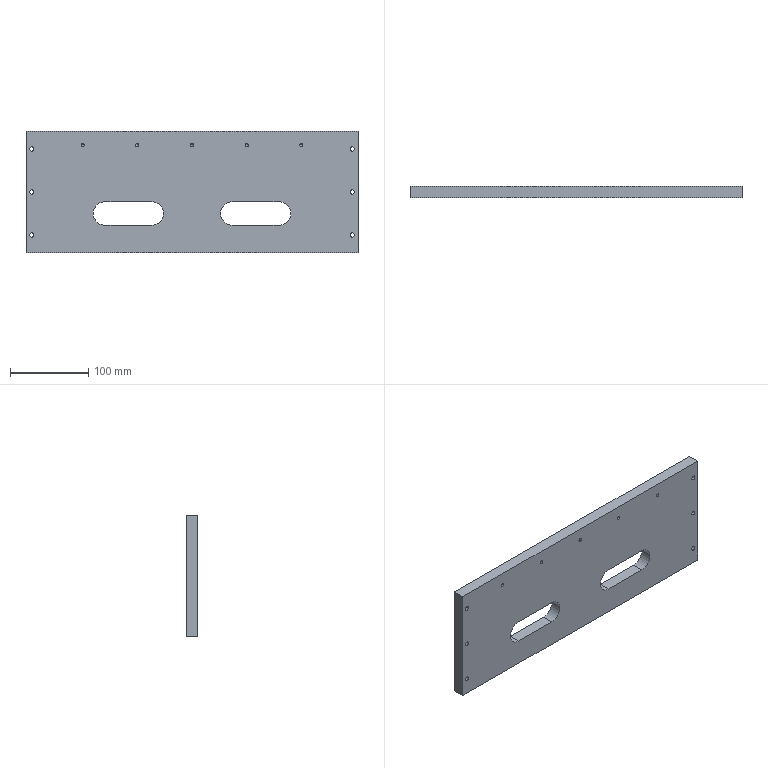Part | STEP file | Rear side plate | 1 solid | 74 faces | box 425 x 15 x 155 mm | volume 907498 mm3 | cylinder 44 | plane 16 | cone 14 | commonest cylinder face diameters 5.5 x12 10 x12 4.2 x10 30 x6 5 x4